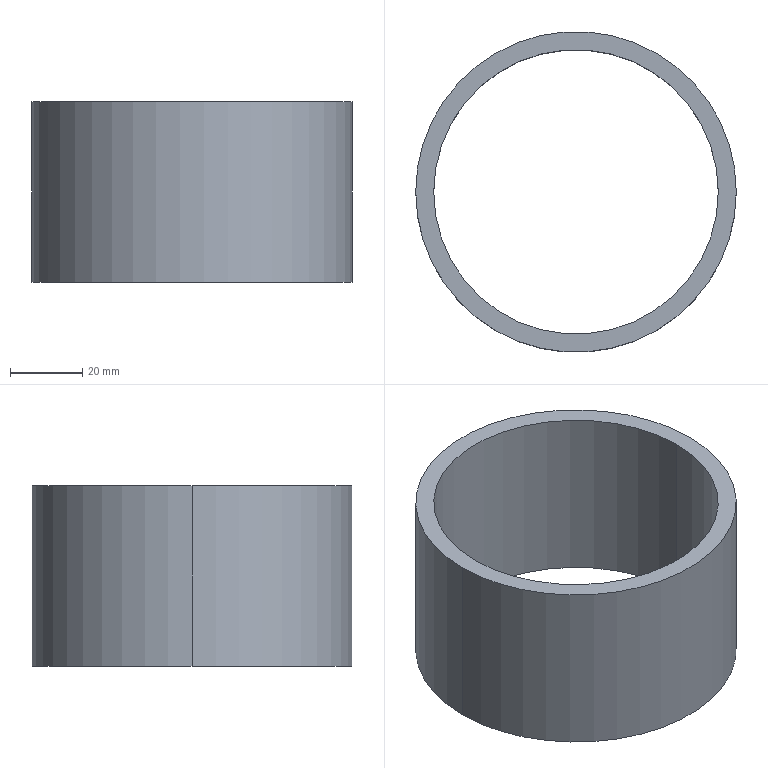Part | SolidWorks | features Extrusion 1 | 1 solid | 6 faces | box 89 x 89 x 50 mm | volume 65973 mm3 | cylinder 4 | plane 2 | commonest cylinder face diameters 79 x2 89 x2
STEP:
#1=CARTESIAN_POINT('',(-39.5,0.,50.));
#2=VERTEX_POINT('',#1);
#3=CARTESIAN_POINT('',(39.5,0.,50.));
#4=VERTEX_POINT('',#3);
#5=CARTESIAN_POINT('',(0.,0.,50.));
#6=DIRECTION('',(0.,0.,1.));
#7=DIRECTION('',(1.,0.,0.));
#8=AXIS2_PLACEMENT_3D('',#5,#6,#7);
#9=CIRCLE('',#8,39.5);
#10=EDGE_CURVE('',#2,#4,#9,.T.);
#11=ORIENTED_EDGE('',*,*,#10,.T.);
#12=CARTESIAN_POINT('',(39.5,0.,0.));
#13=VERTEX_POINT('',#12);
#14=CARTESIAN_POINT('',(39.5,0.,50.));
#15=DIRECTION('',(0.,0.,-1.));
#16=VECTOR('',#15,1000.);
#17=LINE('',#14,#16);
#18=EDGE_CURVE('',#4,#13,#17,.T.);
#19=ORIENTED_EDGE('',*,*,#18,.T.);
#20=CARTESIAN_POINT('',(-39.5,0.,0.));
#21=VERTEX_POINT('',#20);
#22=CARTESIAN_POINT('',(0.,0.,0.));
#23=DIRECTION('',(0.,0.,1.));
#24=DIRECTION('',(1.,0.,0.));
#25=AXIS2_PLACEMENT_3D('',#22,#23,#24);
#26=CIRCLE('',#25,39.5);
#27=EDGE_CURVE('',#21,#13,#26,.T.);
#28=ORIENTED_EDGE('',*,*,#27,.F.);
#29=CARTESIAN_POINT('',(-39.5,0.,50.));
#30=DIRECTION('',(0.,0.,-1.));
#31=VECTOR('',#30,1000.);
#32=LINE('',#29,#31);
#33=EDGE_CURVE('',#2,#21,#32,.T.);
#34=ORIENTED_EDGE('',*,*,#33,.F.);
#35=EDGE_LOOP('',(#11,#19,#28,#34));
#36=FACE_OUTER_BOUND('',#35,.T.);
#37=CARTESIAN_POINT('',(0.,0.,50.));
#38=DIRECTION('',(0.,0.,-1.));
#39=DIRECTION('',(-1.,0.,0.));
#40=AXIS2_PLACEMENT_3D('',#37,#38,#39);
#41=CYLINDRICAL_SURFACE('',#40,39.5);
#42=ADVANCED_FACE('',(#36),#41,.F.);
#43=CARTESIAN_POINT('',(44.5,0.,50.));
#44=VERTEX_POINT('',#43);
#45=CARTESIAN_POINT('',(-44.5,0.,50.));
#46=VERTEX_POINT('',#45);
#47=CARTESIAN_POINT('',(0.,0.,50.));
#48=DIRECTION('',(0.,0.,1.));
#49=DIRECTION('',(1.,0.,0.));
#50=AXIS2_PLACEMENT_3D('',#47,#48,#49);
#51=CIRCLE('',#50,44.5);
#52=EDGE_CURVE('',#44,#46,#51,.T.);
#53=ORIENTED_EDGE('',*,*,#52,.F.);
#54=CARTESIAN_POINT('',(44.5,0.,0.));
#55=VERTEX_POINT('',#54);
#56=CARTESIAN_POINT('',(44.5,0.,50.));
#57=DIRECTION('',(0.,0.,-1.));
#58=VECTOR('',#57,1000.);
#59=LINE('',#56,#58);
#60=EDGE_CURVE('',#44,#55,#59,.T.);
#61=ORIENTED_EDGE('',*,*,#60,.T.);
#62=CARTESIAN_POINT('',(-44.5,0.,0.));
#63=VERTEX_POINT('',#62);
#64=CARTESIAN_POINT('',(0.,0.,0.));
#65=DIRECTION('',(0.,0.,1.));
#66=DIRECTION('',(1.,0.,0.));
#67=AXIS2_PLACEMENT_3D('',#64,#65,#66);
#68=CIRCLE('',#67,44.5);
#69=EDGE_CURVE('',#55,#63,#68,.T.);
#70=ORIENTED_EDGE('',*,*,#69,.T.);
#71=CARTESIAN_POINT('',(-44.5,0.,50.));
#72=DIRECTION('',(0.,0.,-1.));
#73=VECTOR('',#72,1000.);
#74=LINE('',#71,#73);
#75=EDGE_CURVE('',#46,#63,#74,.T.);
#76=ORIENTED_EDGE('',*,*,#75,.F.);
#77=EDGE_LOOP('',(#53,#61,#70,#76));
#78=FACE_OUTER_BOUND('',#77,.T.);
#79=CARTESIAN_POINT('',(0.,0.,50.));
#80=DIRECTION('',(0.,0.,-1.));
#81=DIRECTION('',(-1.,0.,0.));
#82=AXIS2_PLACEMENT_3D('',#79,#80,#81);
#83=CYLINDRICAL_SURFACE('',#82,44.5);
#84=ADVANCED_FACE('',(#78),#83,.T.);
#85=CARTESIAN_POINT('',(0.,0.,50.));
#86=DIRECTION('',(0.,0.,1.));
#87=DIRECTION('',(1.,0.,0.));
#88=AXIS2_PLACEMENT_3D('',#85,#86,#87);
#89=CIRCLE('',#88,44.5);
#90=EDGE_CURVE('',#46,#44,#89,.T.);
#91=ORIENTED_EDGE('',*,*,#90,.T.);
#92=ORIENTED_EDGE('',*,*,#52,.T.);
#93=EDGE_LOOP('',(#91,#92));
#94=FACE_OUTER_BOUND('',#93,.T.);
#95=ORIENTED_EDGE('',*,*,#10,.F.);
#96=CARTESIAN_POINT('',(0.,0.,50.));
#97=DIRECTION('',(0.,0.,1.));
#98=DIRECTION('',(1.,0.,0.));
#99=AXIS2_PLACEMENT_3D('',#96,#97,#98);
#100=CIRCLE('',#99,39.5);
#101=EDGE_CURVE('',#4,#2,#100,.T.);
#102=ORIENTED_EDGE('',*,*,#101,.F.);
#103=EDGE_LOOP('',(#95,#102));
#104=FACE_BOUND('',#103,.T.);
#105=CARTESIAN_POINT('',(0.,0.,50.));
#106=DIRECTION('',(0.,0.,1.));
#107=DIRECTION('',(1.,0.,0.));
#108=AXIS2_PLACEMENT_3D('',#105,#106,#107);
#109=PLANE('',#108);
#110=ADVANCED_FACE('',(#94,#104),#109,.T.);
#111=CARTESIAN_POINT('',(0.,0.,0.));
#112=DIRECTION('',(0.,0.,1.));
#113=DIRECTION('',(1.,0.,0.));
#114=AXIS2_PLACEMENT_3D('',#111,#112,#113);
#115=CIRCLE('',#114,44.5);
#116=EDGE_CURVE('',#63,#55,#115,.T.);
#117=ORIENTED_EDGE('',*,*,#116,.F.);
#118=ORIENTED_EDGE('',*,*,#69,.F.);
#119=EDGE_LOOP('',(#117,#118));
#120=FACE_OUTER_BOUND('',#119,.T.);
#121=ORIENTED_EDGE('',*,*,#27,.T.);
#122=CARTESIAN_POINT('',(0.,0.,0.));
#123=DIRECTION('',(0.,0.,1.));
#124=DIRECTION('',(1.,0.,0.));
#125=AXIS2_PLACEMENT_3D('',#122,#123,#124);
#126=CIRCLE('',#125,39.5);
#127=EDGE_CURVE('',#13,#21,#126,.T.);
#128=ORIENTED_EDGE('',*,*,#127,.T.);
#129=EDGE_LOOP('',(#121,#128));
#130=FACE_BOUND('',#129,.T.);
#131=CARTESIAN_POINT('',(0.,0.,0.));
#132=DIRECTION('',(0.,0.,1.));
#133=DIRECTION('',(1.,0.,0.));
#134=AXIS2_PLACEMENT_3D('',#131,#132,#133);
#135=PLANE('',#134);
#136=ADVANCED_FACE('',(#120,#130),#135,.F.);
#137=ORIENTED_EDGE('',*,*,#60,.F.);
#138=ORIENTED_EDGE('',*,*,#90,.F.);
#139=ORIENTED_EDGE('',*,*,#75,.T.);
#140=ORIENTED_EDGE('',*,*,#116,.T.);
#141=EDGE_LOOP('',(#137,#138,#139,#140));
#142=FACE_OUTER_BOUND('',#141,.T.);
#143=CARTESIAN_POINT('',(0.,0.,50.));
#144=DIRECTION('',(0.,0.,-1.));
#145=DIRECTION('',(-1.,0.,0.));
#146=AXIS2_PLACEMENT_3D('',#143,#144,#145);
#147=CYLINDRICAL_SURFACE('',#146,44.5);
#148=ADVANCED_FACE('',(#142),#147,.T.);
#149=ORIENTED_EDGE('',*,*,#18,.F.);
#150=ORIENTED_EDGE('',*,*,#101,.T.);
#151=ORIENTED_EDGE('',*,*,#33,.T.);
#152=ORIENTED_EDGE('',*,*,#127,.F.);
#153=EDGE_LOOP('',(#149,#150,#151,#152));
#154=FACE_OUTER_BOUND('',#153,.T.);
#155=CARTESIAN_POINT('',(0.,0.,50.));
#156=DIRECTION('',(0.,0.,-1.));
#157=DIRECTION('',(-1.,0.,0.));
#158=AXIS2_PLACEMENT_3D('',#155,#156,#157);
#159=CYLINDRICAL_SURFACE('',#158,39.5);
#160=ADVANCED_FACE('',(#154),#159,.F.);
#161=CLOSED_SHELL('',(#42,#84,#110,#136,#148,#160));
#162=MANIFOLD_SOLID_BREP('',#161);
#163=CARTESIAN_POINT('',(0.,0.,0.));
#164=DIRECTION('',(0.,0.,1.));
#165=DIRECTION('',(1.,0.,0.));
#166=AXIS2_PLACEMENT_3D('',#163,#164,#165);
#167=(LENGTH_UNIT()NAMED_UNIT(*)SI_UNIT(.MILLI.,.METRE.));
#168=UNCERTAINTY_MEASURE_WITH_UNIT(LENGTH_MEASURE(0.00001),#167,'','');
#169=(NAMED_UNIT(*)PLANE_ANGLE_UNIT()SI_UNIT($,.RADIAN.));
#170=(NAMED_UNIT(*)SI_UNIT($,.STERADIAN.)SOLID_ANGLE_UNIT());
#171=(GEOMETRIC_REPRESENTATION_CONTEXT(3)GLOBAL_UNCERTAINTY_ASSIGNED_CONTEXT((#168))GLOBAL_UNIT_ASSIGNED_CONTEXT((#167,#169,#170))REPRESENTATION_CONTEXT('',''));
#172=ADVANCED_BREP_SHAPE_REPRESENTATION('',(#162,#166),#171);